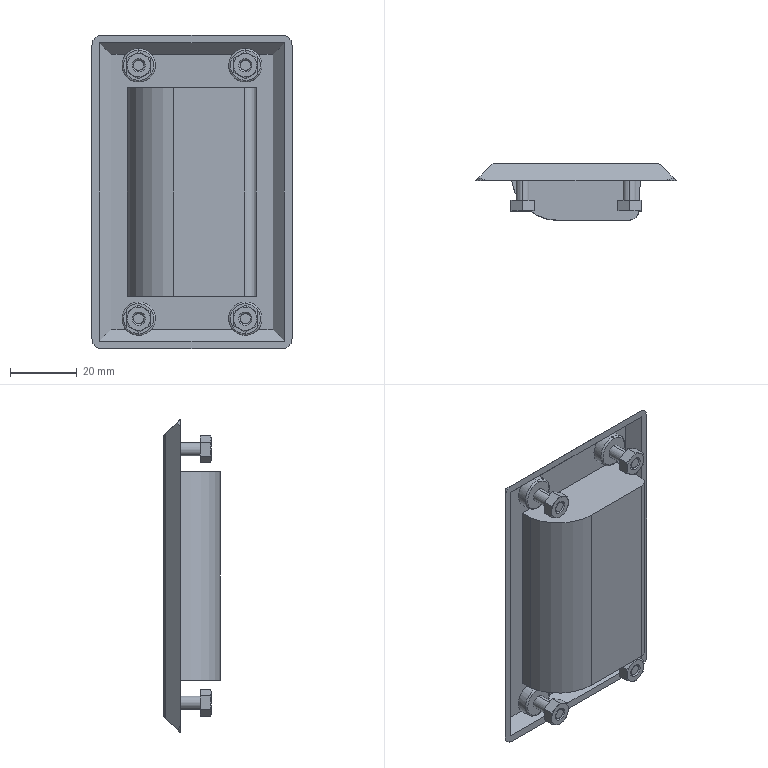Part | NX | features BREP 1 | 1 solid | 146 faces | box 60 x 17 x 94 mm | volume 12686 mm3 | plane 63 | cone 44 | cylinder 31 | torus 8 | commonest cylinder face diameters 4 x11 10 x8 1 x5 6 x5 26 x1 28 x1